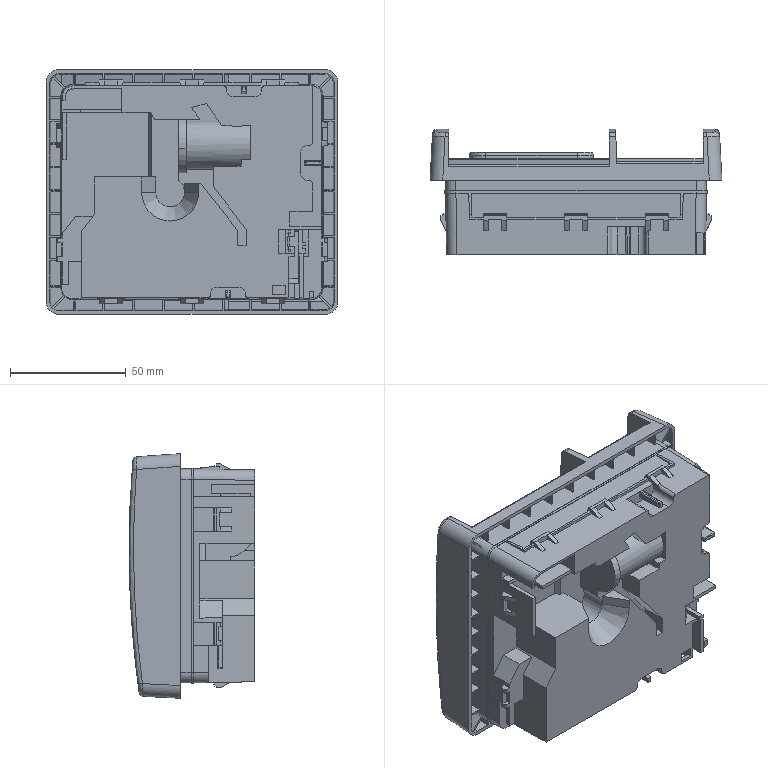Part | STEP file | ZXW735-L-95-02 | 1 solid | 685 faces | box 126.104 x 54.391 x 105.677 mm | volume 392404 mm3 | plane 546 | cylinder 109 | spline 20 | cone 6 | torus 4 | commonest cylinder face diameters 1 x11 0.6 x9 0.4 x8 4 x8 7.8 x8 9 x8